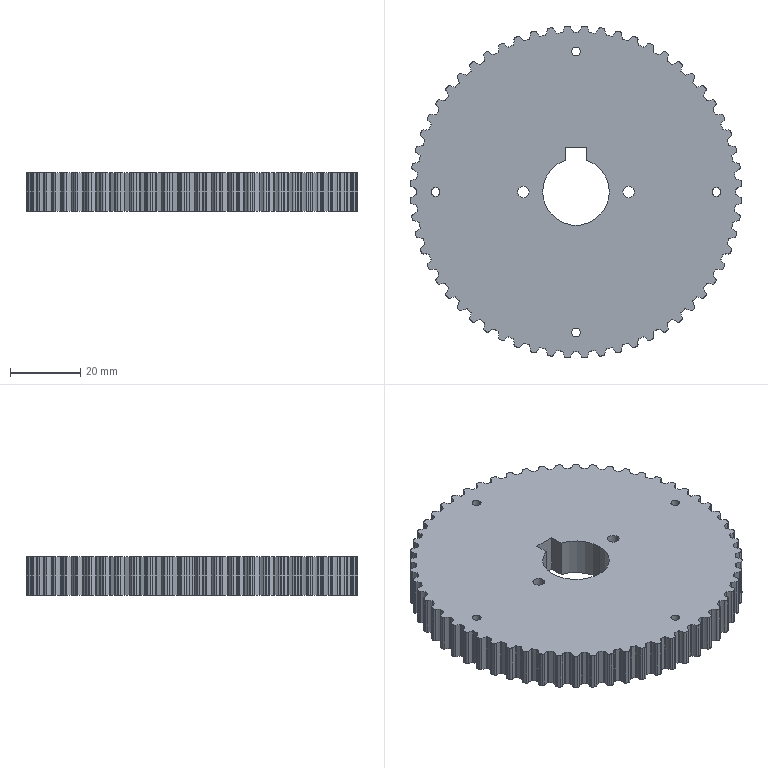Part | STEP file | EBJ01-S5M100-60-A-H-d14 twist motor main pulley SGN-4-02 | 1 solid | 553 faces | box 94.44 x 94.44 x 11 mm | volume 70354 mm3 | cylinder 548 | plane 5 | commonest cylinder face diameters 1.1 x146 0.5 x138 6.55 x128 90.99 x61 94.53 x60 2.5 x8